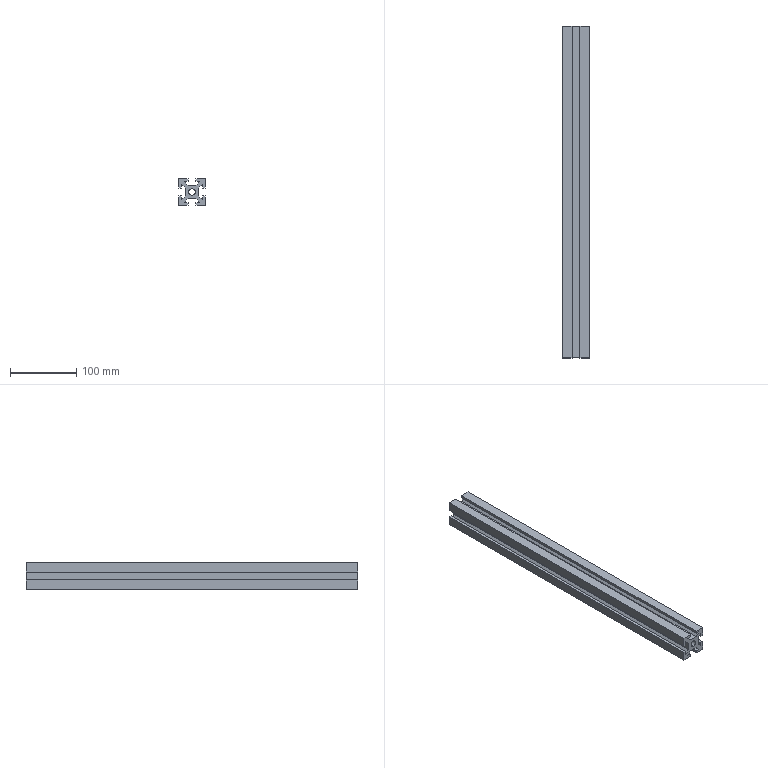Part | SolidWorks | features Extrusion 1 | 1 solid | 40 faces | box 40 x 500 x 40 mm | volume 454553 mm3 | plane 38 | cylinder 2 | commonest cylinder face diameters 10 x2
STEP:
#1=CARTESIAN_POINT('',(0.,500.,-5.));
#2=VERTEX_POINT('',#1);
#3=CARTESIAN_POINT('',(0.,500.,5.));
#4=VERTEX_POINT('',#3);
#5=CARTESIAN_POINT('',(0.,500.,0.));
#6=DIRECTION('',(0.,1.,0.));
#7=DIRECTION('',(0.,0.,1.));
#8=AXIS2_PLACEMENT_3D('',#5,#6,#7);
#9=CIRCLE('',#8,5.);
#10=EDGE_CURVE('',#2,#4,#9,.T.);
#11=ORIENTED_EDGE('',*,*,#10,.T.);
#12=CARTESIAN_POINT('',(0.,0.,5.));
#13=VERTEX_POINT('',#12);
#14=CARTESIAN_POINT('',(0.,500.,5.));
#15=DIRECTION('',(0.,-1.,0.));
#16=VECTOR('',#15,1000.);
#17=LINE('',#14,#16);
#18=EDGE_CURVE('',#4,#13,#17,.T.);
#19=ORIENTED_EDGE('',*,*,#18,.T.);
#20=CARTESIAN_POINT('',(0.,0.,-5.));
#21=VERTEX_POINT('',#20);
#22=CARTESIAN_POINT('',(0.,0.,0.));
#23=DIRECTION('',(0.,1.,0.));
#24=DIRECTION('',(0.,0.,1.));
#25=AXIS2_PLACEMENT_3D('',#22,#23,#24);
#26=CIRCLE('',#25,5.);
#27=EDGE_CURVE('',#21,#13,#26,.T.);
#28=ORIENTED_EDGE('',*,*,#27,.F.);
#29=CARTESIAN_POINT('',(0.,500.,-5.));
#30=DIRECTION('',(0.,-1.,0.));
#31=VECTOR('',#30,1000.);
#32=LINE('',#29,#31);
#33=EDGE_CURVE('',#2,#21,#32,.T.);
#34=ORIENTED_EDGE('',*,*,#33,.F.);
#35=EDGE_LOOP('',(#11,#19,#28,#34));
#36=FACE_OUTER_BOUND('',#35,.T.);
#37=CARTESIAN_POINT('',(0.,500.,0.));
#38=DIRECTION('',(0.,-1.,0.));
#39=DIRECTION('',(0.,0.,-1.));
#40=AXIS2_PLACEMENT_3D('',#37,#38,#39);
#41=CYLINDRICAL_SURFACE('',#40,5.);
#42=ADVANCED_FACE('',(#36),#41,.F.);
#43=CARTESIAN_POINT('',(6.,500.,20.));
#44=VERTEX_POINT('',#43);
#45=CARTESIAN_POINT('',(20.,500.,20.));
#46=VERTEX_POINT('',#45);
#47=CARTESIAN_POINT('',(6.,500.,20.));
#48=DIRECTION('',(1.,0.,0.));
#49=VECTOR('',#48,1000.);
#50=LINE('',#47,#49);
#51=EDGE_CURVE('',#44,#46,#50,.T.);
#52=ORIENTED_EDGE('',*,*,#51,.T.);
#53=CARTESIAN_POINT('',(20.,500.,6.));
#54=VERTEX_POINT('',#53);
#55=CARTESIAN_POINT('',(20.,500.,6.));
#56=DIRECTION('',(0.,0.,-1.));
#57=VECTOR('',#56,1000.);
#58=LINE('',#55,#57);
#59=EDGE_CURVE('',#46,#54,#58,.T.);
#60=ORIENTED_EDGE('',*,*,#59,.T.);
#61=CARTESIAN_POINT('',(16.,500.,6.));
#62=VERTEX_POINT('',#61);
#63=CARTESIAN_POINT('',(16.,500.,6.));
#64=DIRECTION('',(-1.,0.,0.));
#65=VECTOR('',#64,1000.);
#66=LINE('',#63,#65);
#67=EDGE_CURVE('',#54,#62,#66,.T.);
#68=ORIENTED_EDGE('',*,*,#67,.T.);
#69=CARTESIAN_POINT('',(16.,500.,11.757));
#70=VERTEX_POINT('',#69);
#71=CARTESIAN_POINT('',(16.,500.,11.757));
#72=DIRECTION('',(0.,0.,1.));
#73=VECTOR('',#72,1000.);
#74=LINE('',#71,#73);
#75=EDGE_CURVE('',#62,#70,#74,.T.);
#76=ORIENTED_EDGE('',*,*,#75,.T.);
#77=CARTESIAN_POINT('',(10.,500.,5.757));
#78=VERTEX_POINT('',#77);
#79=CARTESIAN_POINT('',(10.,500.,5.757));
#80=DIRECTION('',(-0.7071,0.,-0.7071));
#81=VECTOR('',#80,1000.);
#82=LINE('',#79,#81);
#83=EDGE_CURVE('',#70,#78,#82,.T.);
#84=ORIENTED_EDGE('',*,*,#83,.T.);
#85=CARTESIAN_POINT('',(10.,500.,-5.757));
#86=VERTEX_POINT('',#85);
#87=CARTESIAN_POINT('',(10.,500.,5.757));
#88=DIRECTION('',(0.,0.,-1.));
#89=VECTOR('',#88,1000.);
#90=LINE('',#87,#89);
#91=EDGE_CURVE('',#78,#86,#90,.T.);
#92=ORIENTED_EDGE('',*,*,#91,.T.);
#93=CARTESIAN_POINT('',(16.,500.,-11.757));
#94=VERTEX_POINT('',#93);
#95=CARTESIAN_POINT('',(16.,500.,-11.757));
#96=DIRECTION('',(0.7071,0.,-0.7071));
#97=VECTOR('',#96,1000.);
#98=LINE('',#95,#97);
#99=EDGE_CURVE('',#86,#94,#98,.T.);
#100=ORIENTED_EDGE('',*,*,#99,.T.);
#101=CARTESIAN_POINT('',(16.,500.,-6.));
#102=VERTEX_POINT('',#101);
#103=CARTESIAN_POINT('',(16.,500.,-6.));
#104=DIRECTION('',(0.,0.,1.));
#105=VECTOR('',#104,1000.);
#106=LINE('',#103,#105);
#107=EDGE_CURVE('',#94,#102,#106,.T.);
#108=ORIENTED_EDGE('',*,*,#107,.T.);
#109=CARTESIAN_POINT('',(20.,500.,-6.));
#110=VERTEX_POINT('',#109);
#111=CARTESIAN_POINT('',(20.,500.,-6.));
#112=DIRECTION('',(1.,0.,0.));
#113=VECTOR('',#112,1000.);
#114=LINE('',#111,#113);
#115=EDGE_CURVE('',#102,#110,#114,.T.);
#116=ORIENTED_EDGE('',*,*,#115,.T.);
#117=CARTESIAN_POINT('',(20.,500.,-20.));
#118=VERTEX_POINT('',#117);
#119=CARTESIAN_POINT('',(20.,500.,-20.));
#120=DIRECTION('',(0.,0.,-1.));
#121=VECTOR('',#120,1000.);
#122=LINE('',#119,#121);
#123=EDGE_CURVE('',#110,#118,#122,.T.);
#124=ORIENTED_EDGE('',*,*,#123,.T.);
#125=CARTESIAN_POINT('',(6.,500.,-20.));
#126=VERTEX_POINT('',#125);
#127=CARTESIAN_POINT('',(6.,500.,-20.));
#128=DIRECTION('',(-1.,0.,0.));
#129=VECTOR('',#128,1000.);
#130=LINE('',#127,#129);
#131=EDGE_CURVE('',#118,#126,#130,.T.);
#132=ORIENTED_EDGE('',*,*,#131,.T.);
#133=CARTESIAN_POINT('',(6.,500.,-16.));
#134=VERTEX_POINT('',#133);
#135=CARTESIAN_POINT('',(6.,500.,-16.));
#136=DIRECTION('',(0.,0.,1.));
#137=VECTOR('',#136,1000.);
#138=LINE('',#135,#137);
#139=EDGE_CURVE('',#126,#134,#138,.T.);
#140=ORIENTED_EDGE('',*,*,#139,.T.);
#141=CARTESIAN_POINT('',(11.757,500.,-16.));
#142=VERTEX_POINT('',#141);
#143=CARTESIAN_POINT('',(11.757,500.,-16.));
#144=DIRECTION('',(1.,0.,0.));
#145=VECTOR('',#144,1000.);
#146=LINE('',#143,#145);
#147=EDGE_CURVE('',#134,#142,#146,.T.);
#148=ORIENTED_EDGE('',*,*,#147,.T.);
#149=CARTESIAN_POINT('',(5.757,500.,-10.));
#150=VERTEX_POINT('',#149);
#151=CARTESIAN_POINT('',(5.757,500.,-10.));
#152=DIRECTION('',(-0.7071,0.,0.7071));
#153=VECTOR('',#152,1000.);
#154=LINE('',#151,#153);
#155=EDGE_CURVE('',#142,#150,#154,.T.);
#156=ORIENTED_EDGE('',*,*,#155,.T.);
#157=CARTESIAN_POINT('',(-5.757,500.,-10.));
#158=VERTEX_POINT('',#157);
#159=CARTESIAN_POINT('',(-5.757,500.,-10.));
#160=DIRECTION('',(-1.,0.,0.));
#161=VECTOR('',#160,1000.);
#162=LINE('',#159,#161);
#163=EDGE_CURVE('',#150,#158,#162,.T.);
#164=ORIENTED_EDGE('',*,*,#163,.T.);
#165=CARTESIAN_POINT('',(-11.757,500.,-16.));
#166=VERTEX_POINT('',#165);
#167=CARTESIAN_POINT('',(-11.757,500.,-16.));
#168=DIRECTION('',(-0.7071,0.,-0.7071));
#169=VECTOR('',#168,1000.);
#170=LINE('',#167,#169);
#171=EDGE_CURVE('',#158,#166,#170,.T.);
#172=ORIENTED_EDGE('',*,*,#171,.T.);
#173=CARTESIAN_POINT('',(-6.,500.,-16.));
#174=VERTEX_POINT('',#173);
#175=CARTESIAN_POINT('',(-6.,500.,-16.));
#176=DIRECTION('',(1.,0.,0.));
#177=VECTOR('',#176,1000.);
#178=LINE('',#175,#177);
#179=EDGE_CURVE('',#166,#174,#178,.T.);
#180=ORIENTED_EDGE('',*,*,#179,.T.);
#181=CARTESIAN_POINT('',(-6.,500.,-20.));
#182=VERTEX_POINT('',#181);
#183=CARTESIAN_POINT('',(-6.,500.,-20.));
#184=DIRECTION('',(0.,0.,-1.));
#185=VECTOR('',#184,1000.);
#186=LINE('',#183,#185);
#187=EDGE_CURVE('',#174,#182,#186,.T.);
#188=ORIENTED_EDGE('',*,*,#187,.T.);
#189=CARTESIAN_POINT('',(-20.,500.,-20.));
#190=VERTEX_POINT('',#189);
#191=CARTESIAN_POINT('',(-20.,500.,-20.));
#192=DIRECTION('',(-1.,0.,0.));
#193=VECTOR('',#192,1000.);
#194=LINE('',#191,#193);
#195=EDGE_CURVE('',#182,#190,#194,.T.);
#196=ORIENTED_EDGE('',*,*,#195,.T.);
#197=CARTESIAN_POINT('',(-20.,500.,-6.));
#198=VERTEX_POINT('',#197);
#199=CARTESIAN_POINT('',(-20.,500.,-20.));
#200=DIRECTION('',(0.,0.,1.));
#201=VECTOR('',#200,1000.);
#202=LINE('',#199,#201);
#203=EDGE_CURVE('',#190,#198,#202,.T.);
#204=ORIENTED_EDGE('',*,*,#203,.T.);
#205=CARTESIAN_POINT('',(-16.,500.,-6.));
#206=VERTEX_POINT('',#205);
#207=CARTESIAN_POINT('',(-16.,500.,-6.));
#208=DIRECTION('',(1.,0.,0.));
#209=VECTOR('',#208,1000.);
#210=LINE('',#207,#209);
#211=EDGE_CURVE('',#198,#206,#210,.T.);
#212=ORIENTED_EDGE('',*,*,#211,.T.);
#213=CARTESIAN_POINT('',(-16.,500.,-11.757));
#214=VERTEX_POINT('',#213);
#215=CARTESIAN_POINT('',(-16.,500.,-11.757));
#216=DIRECTION('',(0.,0.,-1.));
#217=VECTOR('',#216,1000.);
#218=LINE('',#215,#217);
#219=EDGE_CURVE('',#206,#214,#218,.T.);
#220=ORIENTED_EDGE('',*,*,#219,.T.);
#221=CARTESIAN_POINT('',(-10.,500.,-5.757));
#222=VERTEX_POINT('',#221);
#223=CARTESIAN_POINT('',(-10.,500.,-5.757));
#224=DIRECTION('',(0.7071,0.,0.7071));
#225=VECTOR('',#224,1000.);
#226=LINE('',#223,#225);
#227=EDGE_CURVE('',#214,#222,#226,.T.);
#228=ORIENTED_EDGE('',*,*,#227,.T.);
#229=CARTESIAN_POINT('',(-10.,500.,5.757));
#230=VERTEX_POINT('',#229);
#231=CARTESIAN_POINT('',(-10.,500.,5.757));
#232=DIRECTION('',(0.,0.,1.));
#233=VECTOR('',#232,1000.);
#234=LINE('',#231,#233);
#235=EDGE_CURVE('',#222,#230,#234,.T.);
#236=ORIENTED_EDGE('',*,*,#235,.T.);
#237=CARTESIAN_POINT('',(-16.,500.,11.757));
#238=VERTEX_POINT('',#237);
#239=CARTESIAN_POINT('',(-16.,500.,11.757));
#240=DIRECTION('',(-0.7071,0.,0.7071));
#241=VECTOR('',#240,1000.);
#242=LINE('',#239,#241);
#243=EDGE_CURVE('',#230,#238,#242,.T.);
#244=ORIENTED_EDGE('',*,*,#243,.T.);
#245=CARTESIAN_POINT('',(-16.,500.,6.));
#246=VERTEX_POINT('',#245);
#247=CARTESIAN_POINT('',(-16.,500.,6.));
#248=DIRECTION('',(0.,0.,-1.));
#249=VECTOR('',#248,1000.);
#250=LINE('',#247,#249);
#251=EDGE_CURVE('',#238,#246,#250,.T.);
#252=ORIENTED_EDGE('',*,*,#251,.T.);
#253=CARTESIAN_POINT('',(-20.,500.,6.));
#254=VERTEX_POINT('',#253);
#255=CARTESIAN_POINT('',(-20.,500.,6.));
#256=DIRECTION('',(-1.,0.,0.));
#257=VECTOR('',#256,1000.);
#258=LINE('',#255,#257);
#259=EDGE_CURVE('',#246,#254,#258,.T.);
#260=ORIENTED_EDGE('',*,*,#259,.T.);
#261=CARTESIAN_POINT('',(-20.,500.,20.));
#262=VERTEX_POINT('',#261);
#263=CARTESIAN_POINT('',(-20.,500.,6.));
#264=DIRECTION('',(0.,0.,1.));
#265=VECTOR('',#264,1000.);
#266=LINE('',#263,#265);
#267=EDGE_CURVE('',#254,#262,#266,.T.);
#268=ORIENTED_EDGE('',*,*,#267,.T.);
#269=CARTESIAN_POINT('',(-6.,500.,20.));
#270=VERTEX_POINT('',#269);
#271=CARTESIAN_POINT('',(-20.,500.,20.));
#272=DIRECTION('',(1.,0.,0.));
#273=VECTOR('',#272,1000.);
#274=LINE('',#271,#273);
#275=EDGE_CURVE('',#262,#270,#274,.T.);
#276=ORIENTED_EDGE('',*,*,#275,.T.);
#277=CARTESIAN_POINT('',(-6.,500.,16.));
#278=VERTEX_POINT('',#277);
#279=CARTESIAN_POINT('',(-6.,500.,16.));
#280=DIRECTION('',(0.,0.,-1.));
#281=VECTOR('',#280,1000.);
#282=LINE('',#279,#281);
#283=EDGE_CURVE('',#270,#278,#282,.T.);
#284=ORIENTED_EDGE('',*,*,#283,.T.);
#285=CARTESIAN_POINT('',(-11.757,500.,16.));
#286=VERTEX_POINT('',#285);
#287=CARTESIAN_POINT('',(-11.757,500.,16.));
#288=DIRECTION('',(-1.,0.,0.));
#289=VECTOR('',#288,1000.);
#290=LINE('',#287,#289);
#291=EDGE_CURVE('',#278,#286,#290,.T.);
#292=ORIENTED_EDGE('',*,*,#291,.T.);
#293=CARTESIAN_POINT('',(-5.757,500.,10.));
#294=VERTEX_POINT('',#293);
#295=CARTESIAN_POINT('',(-5.757,500.,10.));
#296=DIRECTION('',(0.7071,0.,-0.7071));
#297=VECTOR('',#296,1000.);
#298=LINE('',#295,#297);
#299=EDGE_CURVE('',#286,#294,#298,.T.);
#300=ORIENTED_EDGE('',*,*,#299,.T.);
#301=CARTESIAN_POINT('',(5.757,500.,10.));
#302=VERTEX_POINT('',#301);
#303=CARTESIAN_POINT('',(-5.757,500.,10.));
#304=DIRECTION('',(1.,0.,0.));
#305=VECTOR('',#304,1000.);
#306=LINE('',#303,#305);
#307=EDGE_CURVE('',#294,#302,#306,.T.);
#308=ORIENTED_EDGE('',*,*,#307,.T.);
#309=CARTESIAN_POINT('',(11.757,500.,16.));
#310=VERTEX_POINT('',#309);
#311=CARTESIAN_POINT('',(11.757,500.,16.));
#312=DIRECTION('',(0.7071,0.,0.7071));
#313=VECTOR('',#312,1000.);
#314=LINE('',#311,#313);
#315=EDGE_CURVE('',#302,#310,#314,.T.);
#316=ORIENTED_EDGE('',*,*,#315,.T.);
#317=CARTESIAN_POINT('',(6.,500.,16.));
#318=VERTEX_POINT('',#317);
#319=CARTESIAN_POINT('',(6.,500.,16.));
#320=DIRECTION('',(-1.,0.,0.));
#321=VECTOR('',#320,1000.);
#322=LINE('',#319,#321);
#323=EDGE_CURVE('',#310,#318,#322,.T.);
#324=ORIENTED_EDGE('',*,*,#323,.T.);
#325=CARTESIAN_POINT('',(6.,500.,20.));
#326=DIRECTION('',(0.,0.,1.));
#327=VECTOR('',#326,1000.);
#328=LINE('',#325,#327);
#329=EDGE_CURVE('',#318,#44,#328,.T.);
#330=ORIENTED_EDGE('',*,*,#329,.T.);
#331=EDGE_LOOP('',(#52,#60,#68,#76,#84,#92,#100,#108,#116,#124,#132,#140,#148,#156,#164,#172,#180,#188,#196,#204,#212,#220,#228,#236,#244,#252,#260,#268,#276,#284,#292,#300,#308,#316,#324,#330));
#332=FACE_OUTER_BOUND('',#331,.T.);
#333=ORIENTED_EDGE('',*,*,#10,.F.);
#334=CARTESIAN_POINT('',(0.,500.,0.));
#335=DIRECTION('',(0.,1.,0.));
#336=DIRECTION('',(0.,0.,1.));
#337=AXIS2_PLACEMENT_3D('',#334,#335,#336);
#338=CIRCLE('',#337,5.);
#339=EDGE_CURVE('',#4,#2,#338,.T.);
#340=ORIENTED_EDGE('',*,*,#339,.F.);
#341=EDGE_LOOP('',(#333,#340));
#342=FACE_BOUND('',#341,.T.);
#343=CARTESIAN_POINT('',(0.,500.,0.));
#344=DIRECTION('',(0.,-1.,0.));
#345=DIRECTION('',(0.,0.,-1.));
#346=AXIS2_PLACEMENT_3D('',#343,#344,#345);
#347=PLANE('',#346);
#348=ADVANCED_FACE('',(#332,#342),#347,.F.);
#349=CARTESIAN_POINT('',(6.,0.,20.));
#350=VERTEX_POINT('',#349);
#351=CARTESIAN_POINT('',(20.,0.,20.));
#352=VERTEX_POINT('',#351);
#353=CARTESIAN_POINT('',(6.,0.,20.));
#354=DIRECTION('',(1.,0.,0.));
#355=VECTOR('',#354,1000.);
#356=LINE('',#353,#355);
#357=EDGE_CURVE('',#350,#352,#356,.T.);
#358=ORIENTED_EDGE('',*,*,#357,.F.);
#359=CARTESIAN_POINT('',(6.,0.,16.));
#360=VERTEX_POINT('',#359);
#361=CARTESIAN_POINT('',(6.,0.,20.));
#362=DIRECTION('',(0.,0.,1.));
#363=VECTOR('',#362,1000.);
#364=LINE('',#361,#363);
#365=EDGE_CURVE('',#360,#350,#364,.T.);
#366=ORIENTED_EDGE('',*,*,#365,.F.);
#367=CARTESIAN_POINT('',(11.757,0.,16.));
#368=VERTEX_POINT('',#367);
#369=CARTESIAN_POINT('',(6.,0.,16.));
#370=DIRECTION('',(-1.,0.,0.));
#371=VECTOR('',#370,1000.);
#372=LINE('',#369,#371);
#373=EDGE_CURVE('',#368,#360,#372,.T.);
#374=ORIENTED_EDGE('',*,*,#373,.F.);
#375=CARTESIAN_POINT('',(5.757,0.,10.));
#376=VERTEX_POINT('',#375);
#377=CARTESIAN_POINT('',(11.757,0.,16.));
#378=DIRECTION('',(0.7071,0.,0.7071));
#379=VECTOR('',#378,1000.);
#380=LINE('',#377,#379);
#381=EDGE_CURVE('',#376,#368,#380,.T.);
#382=ORIENTED_EDGE('',*,*,#381,.F.);
#383=CARTESIAN_POINT('',(-5.757,0.,10.));
#384=VERTEX_POINT('',#383);
#385=CARTESIAN_POINT('',(-5.757,0.,10.));
#386=DIRECTION('',(1.,0.,0.));
#387=VECTOR('',#386,1000.);
#388=LINE('',#385,#387);
#389=EDGE_CURVE('',#384,#376,#388,.T.);
#390=ORIENTED_EDGE('',*,*,#389,.F.);
#391=CARTESIAN_POINT('',(-11.757,0.,16.));
#392=VERTEX_POINT('',#391);
#393=CARTESIAN_POINT('',(-5.757,0.,10.));
#394=DIRECTION('',(0.7071,0.,-0.7071));
#395=VECTOR('',#394,1000.);
#396=LINE('',#393,#395);
#397=EDGE_CURVE('',#392,#384,#396,.T.);
#398=ORIENTED_EDGE('',*,*,#397,.F.);
#399=CARTESIAN_POINT('',(-6.,0.,16.));
#400=VERTEX_POINT('',#399);
#401=CARTESIAN_POINT('',(-11.757,0.,16.));
#402=DIRECTION('',(-1.,0.,0.));
#403=VECTOR('',#402,1000.);
#404=LINE('',#401,#403);
#405=EDGE_CURVE('',#400,#392,#404,.T.);
#406=ORIENTED_EDGE('',*,*,#405,.F.);
#407=CARTESIAN_POINT('',(-6.,0.,20.));
#408=VERTEX_POINT('',#407);
#409=CARTESIAN_POINT('',(-6.,0.,16.));
#410=DIRECTION('',(0.,0.,-1.));
#411=VECTOR('',#410,1000.);
#412=LINE('',#409,#411);
#413=EDGE_CURVE('',#408,#400,#412,.T.);
#414=ORIENTED_EDGE('',*,*,#413,.F.);
#415=CARTESIAN_POINT('',(-20.,0.,20.));
#416=VERTEX_POINT('',#415);
#417=CARTESIAN_POINT('',(-20.,0.,20.));
#418=DIRECTION('',(1.,0.,0.));
#419=VECTOR('',#418,1000.);
#420=LINE('',#417,#419);
#421=EDGE_CURVE('',#416,#408,#420,.T.);
#422=ORIENTED_EDGE('',*,*,#421,.F.);
#423=CARTESIAN_POINT('',(-20.,0.,6.));
#424=VERTEX_POINT('',#423);
#425=CARTESIAN_POINT('',(-20.,0.,6.));
#426=DIRECTION('',(0.,0.,1.));
#427=VECTOR('',#426,1000.);
#428=LINE('',#425,#427);
#429=EDGE_CURVE('',#424,#416,#428,.T.);
#430=ORIENTED_EDGE('',*,*,#429,.F.);
#431=CARTESIAN_POINT('',(-16.,0.,6.));
#432=VERTEX_POINT('',#431);
#433=CARTESIAN_POINT('',(-20.,0.,6.));
#434=DIRECTION('',(-1.,0.,0.));
#435=VECTOR('',#434,1000.);
#436=LINE('',#433,#435);
#437=EDGE_CURVE('',#432,#424,#436,.T.);
#438=ORIENTED_EDGE('',*,*,#437,.F.);
#439=CARTESIAN_POINT('',(-16.,0.,11.757));
#440=VERTEX_POINT('',#439);
#441=CARTESIAN_POINT('',(-16.,0.,6.));
#442=DIRECTION('',(0.,0.,-1.));
#443=VECTOR('',#442,1000.);
#444=LINE('',#441,#443);
#445=EDGE_CURVE('',#440,#432,#444,.T.);
#446=ORIENTED_EDGE('',*,*,#445,.F.);
#447=CARTESIAN_POINT('',(-10.,0.,5.757));
#448=VERTEX_POINT('',#447);
#449=CARTESIAN_POINT('',(-16.,0.,11.757));
#450=DIRECTION('',(-0.7071,0.,0.7071));
#451=VECTOR('',#450,1000.);
#452=LINE('',#449,#451);
#453=EDGE_CURVE('',#448,#440,#452,.T.);
#454=ORIENTED_EDGE('',*,*,#453,.F.);
#455=CARTESIAN_POINT('',(-10.,0.,-5.757));
#456=VERTEX_POINT('',#455);
#457=CARTESIAN_POINT('',(-10.,0.,5.757));
#458=DIRECTION('',(0.,0.,1.));
#459=VECTOR('',#458,1000.);
#460=LINE('',#457,#459);
#461=EDGE_CURVE('',#456,#448,#460,.T.);
#462=ORIENTED_EDGE('',*,*,#461,.F.);
#463=CARTESIAN_POINT('',(-16.,0.,-11.757));
#464=VERTEX_POINT('',#463);
#465=CARTESIAN_POINT('',(-10.,0.,-5.757));
#466=DIRECTION('',(0.7071,0.,0.7071));
#467=VECTOR('',#466,1000.);
#468=LINE('',#465,#467);
#469=EDGE_CURVE('',#464,#456,#468,.T.);
#470=ORIENTED_EDGE('',*,*,#469,.F.);
#471=CARTESIAN_POINT('',(-16.,0.,-6.));
#472=VERTEX_POINT('',#471);
#473=CARTESIAN_POINT('',(-16.,0.,-11.757));
#474=DIRECTION('',(0.,0.,-1.));
#475=VECTOR('',#474,1000.);
#476=LINE('',#473,#475);
#477=EDGE_CURVE('',#472,#464,#476,.T.);
#478=ORIENTED_EDGE('',*,*,#477,.F.);
#479=CARTESIAN_POINT('',(-20.,0.,-6.));
#480=VERTEX_POINT('',#479);
#481=CARTESIAN_POINT('',(-16.,0.,-6.));
#482=DIRECTION('',(1.,0.,0.));
#483=VECTOR('',#482,1000.);
#484=LINE('',#481,#483);
#485=EDGE_CURVE('',#480,#472,#484,.T.);
#486=ORIENTED_EDGE('',*,*,#485,.F.);
#487=CARTESIAN_POINT('',(-20.,0.,-20.));
#488=VERTEX_POINT('',#487);
#489=CARTESIAN_POINT('',(-20.,0.,-20.));
#490=DIRECTION('',(0.,0.,1.));
#491=VECTOR('',#490,1000.);
#492=LINE('',#489,#491);
#493=EDGE_CURVE('',#488,#480,#492,.T.);
#494=ORIENTED_EDGE('',*,*,#493,.F.);
#495=CARTESIAN_POINT('',(-6.,0.,-20.));
#496=VERTEX_POINT('',#495);
#497=CARTESIAN_POINT('',(-20.,0.,-20.));
#498=DIRECTION('',(-1.,0.,0.));
#499=VECTOR('',#498,1000.);
#500=LINE('',#497,#499);
#501=EDGE_CURVE('',#496,#488,#500,.T.);
#502=ORIENTED_EDGE('',*,*,#501,.F.);
#503=CARTESIAN_POINT('',(-6.,0.,-16.));
#504=VERTEX_POINT('',#503);
#505=CARTESIAN_POINT('',(-6.,0.,-20.));
#506=DIRECTION('',(0.,0.,-1.));
#507=VECTOR('',#506,1000.);
#508=LINE('',#505,#507);
#509=EDGE_CURVE('',#504,#496,#508,.T.);
#510=ORIENTED_EDGE('',*,*,#509,.F.);
#511=CARTESIAN_POINT('',(-11.757,0.,-16.));
#512=VERTEX_POINT('',#511);
#513=CARTESIAN_POINT('',(-6.,0.,-16.));
#514=DIRECTION('',(1.,0.,0.));
#515=VECTOR('',#514,1000.);
#516=LINE('',#513,#515);
#517=EDGE_CURVE('',#512,#504,#516,.T.);
#518=ORIENTED_EDGE('',*,*,#517,.F.);
#519=CARTESIAN_POINT('',(-5.757,0.,-10.));
#520=VERTEX_POINT('',#519);
#521=CARTESIAN_POINT('',(-11.757,0.,-16.));
#522=DIRECTION('',(-0.7071,0.,-0.7071));
#523=VECTOR('',#522,1000.);
#524=LINE('',#521,#523);
#525=EDGE_CURVE('',#520,#512,#524,.T.);
#526=ORIENTED_EDGE('',*,*,#525,.F.);
#527=CARTESIAN_POINT('',(5.757,0.,-10.));
#528=VERTEX_POINT('',#527);
#529=CARTESIAN_POINT('',(-5.757,0.,-10.));
#530=DIRECTION('',(-1.,0.,0.));
#531=VECTOR('',#530,1000.);
#532=LINE('',#529,#531);
#533=EDGE_CURVE('',#528,#520,#532,.T.);
#534=ORIENTED_EDGE('',*,*,#533,.F.);
#535=CARTESIAN_POINT('',(11.757,0.,-16.));
#536=VERTEX_POINT('',#535);
#537=CARTESIAN_POINT('',(5.757,0.,-10.));
#538=DIRECTION('',(-0.7071,0.,0.7071));
#539=VECTOR('',#538,1000.);
#540=LINE('',#537,#539);
#541=EDGE_CURVE('',#536,#528,#540,.T.);
#542=ORIENTED_EDGE('',*,*,#541,.F.);
#543=CARTESIAN_POINT('',(6.,0.,-16.));
#544=VERTEX_POINT('',#543);
#545=CARTESIAN_POINT('',(11.757,0.,-16.));
#546=DIRECTION('',(1.,0.,0.));
#547=VECTOR('',#546,1000.);
#548=LINE('',#545,#547);
#549=EDGE_CURVE('',#544,#536,#548,.T.);
#550=ORIENTED_EDGE('',*,*,#549,.F.);
#551=CARTESIAN_POINT('',(6.,0.,-20.));
#552=VERTEX_POINT('',#551);
#553=CARTESIAN_POINT('',(6.,0.,-16.));
#554=DIRECTION('',(0.,0.,1.));
#555=VECTOR('',#554,1000.);
#556=LINE('',#553,#555);
#557=EDGE_CURVE('',#552,#544,#556,.T.);
#558=ORIENTED_EDGE('',*,*,#557,.F.);
#559=CARTESIAN_POINT('',(20.,0.,-20.));
#560=VERTEX_POINT('',#559);
#561=CARTESIAN_POINT('',(6.,0.,-20.));
#562=DIRECTION('',(-1.,0.,0.));
#563=VECTOR('',#562,1000.);
#564=LINE('',#561,#563);
#565=EDGE_CURVE('',#560,#552,#564,.T.);
#566=ORIENTED_EDGE('',*,*,#565,.F.);
#567=CARTESIAN_POINT('',(20.,0.,-6.));
#568=VERTEX_POINT('',#567);
#569=CARTESIAN_POINT('',(20.,0.,-20.));
#570=DIRECTION('',(0.,0.,-1.));
#571=VECTOR('',#570,1000.);
#572=LINE('',#569,#571);
#573=EDGE_CURVE('',#568,#560,#572,.T.);
#574=ORIENTED_EDGE('',*,*,#573,.F.);
#575=CARTESIAN_POINT('',(16.,0.,-6.));
#576=VERTEX_POINT('',#575);
#577=CARTESIAN_POINT('',(20.,0.,-6.));
#578=DIRECTION('',(1.,0.,0.));
#579=VECTOR('',#578,1000.);
#580=LINE('',#577,#579);
#581=EDGE_CURVE('',#576,#568,#580,.T.);
#582=ORIENTED_EDGE('',*,*,#581,.F.);
#583=CARTESIAN_POINT('',(16.,0.,-11.757));
#584=VERTEX_POINT('',#583);
#585=CARTESIAN_POINT('',(16.,0.,-6.));
#586=DIRECTION('',(0.,0.,1.));
#587=VECTOR('',#586,1000.);
#588=LINE('',#585,#587);
#589=EDGE_CURVE('',#584,#576,#588,.T.);
#590=ORIENTED_EDGE('',*,*,#589,.F.);
#591=CARTESIAN_POINT('',(10.,0.,-5.757));
#592=VERTEX_POINT('',#591);
#593=CARTESIAN_POINT('',(16.,0.,-11.757));
#594=DIRECTION('',(0.7071,0.,-0.7071));
#595=VECTOR('',#594,1000.);
#596=LINE('',#593,#595);
#597=EDGE_CURVE('',#592,#584,#596,.T.);
#598=ORIENTED_EDGE('',*,*,#597,.F.);
#599=CARTESIAN_POINT('',(10.,0.,5.757));
#600=VERTEX_POINT('',#599);
#601=CARTESIAN_POINT('',(10.,0.,5.757));
#602=DIRECTION('',(0.,0.,-1.));
#603=VECTOR('',#602,1000.);
#604=LINE('',#601,#603);
#605=EDGE_CURVE('',#600,#592,#604,.T.);
#606=ORIENTED_EDGE('',*,*,#605,.F.);
#607=CARTESIAN_POINT('',(16.,0.,11.757));
#608=VERTEX_POINT('',#607);
#609=CARTESIAN_POINT('',(10.,0.,5.757));
#610=DIRECTION('',(-0.7071,0.,-0.7071));
#611=VECTOR('',#610,1000.);
#612=LINE('',#609,#611);
#613=EDGE_CURVE('',#608,#600,#612,.T.);
#614=ORIENTED_EDGE('',*,*,#613,.F.);
#615=CARTESIAN_POINT('',(16.,0.,6.));
#616=VERTEX_POINT('',#615);
#617=CARTESIAN_POINT('',(16.,0.,11.757));
#618=DIRECTION('',(0.,0.,1.));
#619=VECTOR('',#618,1000.);
#620=LINE('',#617,#619);
#621=EDGE_CURVE('',#616,#608,#620,.T.);
#622=ORIENTED_EDGE('',*,*,#621,.F.);
#623=CARTESIAN_POINT('',(20.,0.,6.));
#624=VERTEX_POINT('',#623);
#625=CARTESIAN_POINT('',(16.,0.,6.));
#626=DIRECTION('',(-1.,0.,0.));
#627=VECTOR('',#626,1000.);
#628=LINE('',#625,#627);
#629=EDGE_CURVE('',#624,#616,#628,.T.);
#630=ORIENTED_EDGE('',*,*,#629,.F.);
#631=CARTESIAN_POINT('',(20.,0.,6.));
#632=DIRECTION('',(0.,0.,-1.));
#633=VECTOR('',#632,1000.);
#634=LINE('',#631,#633);
#635=EDGE_CURVE('',#352,#624,#634,.T.);
#636=ORIENTED_EDGE('',*,*,#635,.F.);
#637=EDGE_LOOP('',(#358,#366,#374,#382,#390,#398,#406,#414,#422,#430,#438,#446,#454,#462,#470,#478,#486,#494,#502,#510,#518,#526,#534,#542,#550,#558,#566,#574,#582,#590,#598,#606,#614,#622,#630,#636));
#638=FACE_OUTER_BOUND('',#637,.T.);
#639=ORIENTED_EDGE('',*,*,#27,.T.);
#640=CARTESIAN_POINT('',(0.,0.,0.));
#641=DIRECTION('',(0.,1.,0.));
#642=DIRECTION('',(0.,0.,1.));
#643=AXIS2_PLACEMENT_3D('',#640,#641,#642);
#644=CIRCLE('',#643,5.);
#645=EDGE_CURVE('',#13,#21,#644,.T.);
#646=ORIENTED_EDGE('',*,*,#645,.T.);
#647=EDGE_LOOP('',(#639,#646));
#648=FACE_BOUND('',#647,.T.);
#649=CARTESIAN_POINT('',(0.,0.,0.));
#650=DIRECTION('',(0.,-1.,0.));
#651=DIRECTION('',(0.,0.,-1.));
#652=AXIS2_PLACEMENT_3D('',#649,#650,#651);
#653=PLANE('',#652);
#654=ADVANCED_FACE('',(#638,#648),#653,.T.);
#655=ORIENTED_EDGE('',*,*,#357,.T.);
#656=CARTESIAN_POINT('',(20.,500.,20.));
#657=DIRECTION('',(0.,-1.,0.));
#658=VECTOR('',#657,1000.);
#659=LINE('',#656,#658);
#660=EDGE_CURVE('',#46,#352,#659,.T.);
#661=ORIENTED_EDGE('',*,*,#660,.F.);
#662=ORIENTED_EDGE('',*,*,#51,.F.);
#663=CARTESIAN_POINT('',(6.,500.,20.));
#664=DIRECTION('',(0.,-1.,0.));
#665=VECTOR('',#664,1000.);
#666=LINE('',#663,#665);
#667=EDGE_CURVE('',#44,#350,#666,.T.);
#668=ORIENTED_EDGE('',*,*,#667,.T.);
#669=EDGE_LOOP('',(#655,#661,#662,#668));
#670=FACE_OUTER_BOUND('',#669,.T.);
#671=CARTESIAN_POINT('',(6.,500.,20.));
#672=DIRECTION('',(0.,0.,-1.));
#673=DIRECTION('',(-1.,0.,0.));
#674=AXIS2_PLACEMENT_3D('',#671,#672,#673);
#675=PLANE('',#674);
#676=ADVANCED_FACE('',(#670),#675,.F.);
#677=ORIENTED_EDGE('',*,*,#635,.T.);
#678=CARTESIAN_POINT('',(20.,500.,6.));
#679=DIRECTION('',(0.,-1.,0.));
#680=VECTOR('',#679,1000.);
#681=LINE('',#678,#680);
#682=EDGE_CURVE('',#54,#624,#681,.T.);
#683=ORIENTED_EDGE('',*,*,#682,.F.);
#684=ORIENTED_EDGE('',*,*,#59,.F.);
#685=ORIENTED_EDGE('',*,*,#660,.T.);
#686=EDGE_LOOP('',(#677,#683,#684,#685));
#687=FACE_OUTER_BOUND('',#686,.T.);
#688=CARTESIAN_POINT('',(20.,500.,6.));
#689=DIRECTION('',(-1.,0.,0.));
#690=DIRECTION('',(0.,0.,1.));
#691=AXIS2_PLACEMENT_3D('',#688,#689,#690);
#692=PLANE('',#691);
#693=ADVANCED_FACE('',(#687),#692,.F.);
#694=ORIENTED_EDGE('',*,*,#629,.T.);
#695=CARTESIAN_POINT('',(16.,500.,6.));
#696=DIRECTION('',(0.,-1.,0.));
#697=VECTOR('',#696,1000.);
#698=LINE('',#695,#697);
#699=EDGE_CURVE('',#62,#616,#698,.T.);
#700=ORIENTED_EDGE('',*,*,#699,.F.);
#701=ORIENTED_EDGE('',*,*,#67,.F.);
#702=ORIENTED_EDGE('',*,*,#682,.T.);
#703=EDGE_LOOP('',(#694,#700,#701,#702));
#704=FACE_OUTER_BOUND('',#703,.T.);
#705=CARTESIAN_POINT('',(16.,500.,6.));
#706=DIRECTION('',(0.,0.,1.));
#707=DIRECTION('',(1.,0.,0.));
#708=AXIS2_PLACEMENT_3D('',#705,#706,#707);
#709=PLANE('',#708);
#710=ADVANCED_FACE('',(#704),#709,.F.);
#711=ORIENTED_EDGE('',*,*,#621,.T.);
#712=CARTESIAN_POINT('',(16.,500.,11.757));
#713=DIRECTION('',(0.,-1.,0.));
#714=VECTOR('',#713,1000.);
#715=LINE('',#712,#714);
#716=EDGE_CURVE('',#70,#608,#715,.T.);
#717=ORIENTED_EDGE('',*,*,#716,.F.);
#718=ORIENTED_EDGE('',*,*,#75,.F.);
#719=ORIENTED_EDGE('',*,*,#699,.T.);
#720=EDGE_LOOP('',(#711,#717,#718,#719));
#721=FACE_OUTER_BOUND('',#720,.T.);
#722=CARTESIAN_POINT('',(16.,500.,11.757));
#723=DIRECTION('',(1.,0.,0.));
#724=DIRECTION('',(0.,0.,-1.));
#725=AXIS2_PLACEMENT_3D('',#722,#723,#724);
#726=PLANE('',#725);
#727=ADVANCED_FACE('',(#721),#726,.F.);
#728=ORIENTED_EDGE('',*,*,#613,.T.);
#729=CARTESIAN_POINT('',(10.,500.,5.757));
#730=DIRECTION('',(0.,-1.,0.));
#731=VECTOR('',#730,1000.);
#732=LINE('',#729,#731);
#733=EDGE_CURVE('',#78,#600,#732,.T.);
#734=ORIENTED_EDGE('',*,*,#733,.F.);
#735=ORIENTED_EDGE('',*,*,#83,.F.);
#736=ORIENTED_EDGE('',*,*,#716,.T.);
#737=EDGE_LOOP('',(#728,#734,#735,#736));
#738=FACE_OUTER_BOUND('',#737,.T.);
#739=CARTESIAN_POINT('',(10.,500.,5.757));
#740=DIRECTION('',(-0.7071,0.,0.7071));
#741=DIRECTION('',(0.7071,0.,0.7071));
#742=AXIS2_PLACEMENT_3D('',#739,#740,#741);
#743=PLANE('',#742);
#744=ADVANCED_FACE('',(#738),#743,.F.);
#745=ORIENTED_EDGE('',*,*,#605,.T.);
#746=CARTESIAN_POINT('',(10.,500.,-5.757));
#747=DIRECTION('',(0.,-1.,0.));
#748=VECTOR('',#747,1000.);
#749=LINE('',#746,#748);
#750=EDGE_CURVE('',#86,#592,#749,.T.);
#751=ORIENTED_EDGE('',*,*,#750,.F.);
#752=ORIENTED_EDGE('',*,*,#91,.F.);
#753=ORIENTED_EDGE('',*,*,#733,.T.);
#754=EDGE_LOOP('',(#745,#751,#752,#753));
#755=FACE_OUTER_BOUND('',#754,.T.);
#756=CARTESIAN_POINT('',(10.,500.,5.757));
#757=DIRECTION('',(-1.,0.,0.));
#758=DIRECTION('',(0.,0.,1.));
#759=AXIS2_PLACEMENT_3D('',#756,#757,#758);
#760=PLANE('',#759);
#761=ADVANCED_FACE('',(#755),#760,.F.);
#762=ORIENTED_EDGE('',*,*,#597,.T.);
#763=CARTESIAN_POINT('',(16.,500.,-11.757));
#764=DIRECTION('',(0.,-1.,0.));
#765=VECTOR('',#764,1000.);
#766=LINE('',#763,#765);
#767=EDGE_CURVE('',#94,#584,#766,.T.);
#768=ORIENTED_EDGE('',*,*,#767,.F.);
#769=ORIENTED_EDGE('',*,*,#99,.F.);
#770=ORIENTED_EDGE('',*,*,#750,.T.);
#771=EDGE_LOOP('',(#762,#768,#769,#770));
#772=FACE_OUTER_BOUND('',#771,.T.);
#773=CARTESIAN_POINT('',(16.,500.,-11.757));
#774=DIRECTION('',(-0.7071,0.,-0.7071));
#775=DIRECTION('',(-0.7071,0.,0.7071));
#776=AXIS2_PLACEMENT_3D('',#773,#774,#775);
#777=PLANE('',#776);
#778=ADVANCED_FACE('',(#772),#777,.F.);
#779=ORIENTED_EDGE('',*,*,#589,.T.);
#780=CARTESIAN_POINT('',(16.,500.,-6.));
#781=DIRECTION('',(0.,-1.,0.));
#782=VECTOR('',#781,1000.);
#783=LINE('',#780,#782);
#784=EDGE_CURVE('',#102,#576,#783,.T.);
#785=ORIENTED_EDGE('',*,*,#784,.F.);
#786=ORIENTED_EDGE('',*,*,#107,.F.);
#787=ORIENTED_EDGE('',*,*,#767,.T.);
#788=EDGE_LOOP('',(#779,#785,#786,#787));
#789=FACE_OUTER_BOUND('',#788,.T.);
#790=CARTESIAN_POINT('',(16.,500.,-6.));
#791=DIRECTION('',(1.,0.,0.));
#792=DIRECTION('',(0.,0.,-1.));
#793=AXIS2_PLACEMENT_3D('',#790,#791,#792);
#794=PLANE('',#793);
#795=ADVANCED_FACE('',(#789),#794,.F.);
#796=ORIENTED_EDGE('',*,*,#581,.T.);
#797=CARTESIAN_POINT('',(20.,500.,-6.));
#798=DIRECTION('',(0.,-1.,0.));
#799=VECTOR('',#798,1000.);
#800=LINE('',#797,#799);
#801=EDGE_CURVE('',#110,#568,#800,.T.);
#802=ORIENTED_EDGE('',*,*,#801,.F.);
#803=ORIENTED_EDGE('',*,*,#115,.F.);
#804=ORIENTED_EDGE('',*,*,#784,.T.);
#805=EDGE_LOOP('',(#796,#802,#803,#804));
#806=FACE_OUTER_BOUND('',#805,.T.);
#807=CARTESIAN_POINT('',(20.,500.,-6.));
#808=DIRECTION('',(0.,0.,-1.));
#809=DIRECTION('',(-1.,0.,0.));
#810=AXIS2_PLACEMENT_3D('',#807,#808,#809);
#811=PLANE('',#810);
#812=ADVANCED_FACE('',(#806),#811,.F.);
#813=ORIENTED_EDGE('',*,*,#573,.T.);
#814=CARTESIAN_POINT('',(20.,500.,-20.));
#815=DIRECTION('',(0.,-1.,0.));
#816=VECTOR('',#815,1000.);
#817=LINE('',#814,#816);
#818=EDGE_CURVE('',#118,#560,#817,.T.);
#819=ORIENTED_EDGE('',*,*,#818,.F.);
#820=ORIENTED_EDGE('',*,*,#123,.F.);
#821=ORIENTED_EDGE('',*,*,#801,.T.);
#822=EDGE_LOOP('',(#813,#819,#820,#821));
#823=FACE_OUTER_BOUND('',#822,.T.);
#824=CARTESIAN_POINT('',(20.,500.,-20.));
#825=DIRECTION('',(-1.,0.,0.));
#826=DIRECTION('',(0.,0.,1.));
#827=AXIS2_PLACEMENT_3D('',#824,#825,#826);
#828=PLANE('',#827);
#829=ADVANCED_FACE('',(#823),#828,.F.);
#830=ORIENTED_EDGE('',*,*,#565,.T.);
#831=CARTESIAN_POINT('',(6.,500.,-20.));
#832=DIRECTION('',(0.,-1.,0.));
#833=VECTOR('',#832,1000.);
#834=LINE('',#831,#833);
#835=EDGE_CURVE('',#126,#552,#834,.T.);
#836=ORIENTED_EDGE('',*,*,#835,.F.);
#837=ORIENTED_EDGE('',*,*,#131,.F.);
#838=ORIENTED_EDGE('',*,*,#818,.T.);
#839=EDGE_LOOP('',(#830,#836,#837,#838));
#840=FACE_OUTER_BOUND('',#839,.T.);
#841=CARTESIAN_POINT('',(6.,500.,-20.));
#842=DIRECTION('',(0.,0.,1.));
#843=DIRECTION('',(1.,0.,0.));
#844=AXIS2_PLACEMENT_3D('',#841,#842,#843);
#845=PLANE('',#844);
#846=ADVANCED_FACE('',(#840),#845,.F.);
#847=ORIENTED_EDGE('',*,*,#557,.T.);
#848=CARTESIAN_POINT('',(6.,500.,-16.));
#849=DIRECTION('',(0.,-1.,0.));
#850=VECTOR('',#849,1000.);
#851=LINE('',#848,#850);
#852=EDGE_CURVE('',#134,#544,#851,.T.);
#853=ORIENTED_EDGE('',*,*,#852,.F.);
#854=ORIENTED_EDGE('',*,*,#139,.F.);
#855=ORIENTED_EDGE('',*,*,#835,.T.);
#856=EDGE_LOOP('',(#847,#853,#854,#855));
#857=FACE_OUTER_BOUND('',#856,.T.);
#858=CARTESIAN_POINT('',(6.,500.,-16.));
#859=DIRECTION('',(1.,0.,0.));
#860=DIRECTION('',(0.,0.,-1.));
#861=AXIS2_PLACEMENT_3D('',#858,#859,#860);
#862=PLANE('',#861);
#863=ADVANCED_FACE('',(#857),#862,.F.);
#864=ORIENTED_EDGE('',*,*,#549,.T.);
#865=CARTESIAN_POINT('',(11.757,500.,-16.));
#866=DIRECTION('',(0.,-1.,0.));
#867=VECTOR('',#866,1000.);
#868=LINE('',#865,#867);
#869=EDGE_CURVE('',#142,#536,#868,.T.);
#870=ORIENTED_EDGE('',*,*,#869,.F.);
#871=ORIENTED_EDGE('',*,*,#147,.F.);
#872=ORIENTED_EDGE('',*,*,#852,.T.);
#873=EDGE_LOOP('',(#864,#870,#871,#872));
#874=FACE_OUTER_BOUND('',#873,.T.);
#875=CARTESIAN_POINT('',(11.757,500.,-16.));
#876=DIRECTION('',(0.,0.,-1.));
#877=DIRECTION('',(-1.,0.,0.));
#878=AXIS2_PLACEMENT_3D('',#875,#876,#877);
#879=PLANE('',#878);
#880=ADVANCED_FACE('',(#874),#879,.F.);
#881=ORIENTED_EDGE('',*,*,#541,.T.);
#882=CARTESIAN_POINT('',(5.757,500.,-10.));
#883=DIRECTION('',(0.,-1.,0.));
#884=VECTOR('',#883,1000.);
#885=LINE('',#882,#884);
#886=EDGE_CURVE('',#150,#528,#885,.T.);
#887=ORIENTED_EDGE('',*,*,#886,.F.);
#888=ORIENTED_EDGE('',*,*,#155,.F.);
#889=ORIENTED_EDGE('',*,*,#869,.T.);
#890=EDGE_LOOP('',(#881,#887,#888,#889));
#891=FACE_OUTER_BOUND('',#890,.T.);
#892=CARTESIAN_POINT('',(5.757,500.,-10.));
#893=DIRECTION('',(0.7071,0.,0.7071));
#894=DIRECTION('',(0.7071,0.,-0.7071));
#895=AXIS2_PLACEMENT_3D('',#892,#893,#894);
#896=PLANE('',#895);
#897=ADVANCED_FACE('',(#891),#896,.F.);
#898=ORIENTED_EDGE('',*,*,#533,.T.);
#899=CARTESIAN_POINT('',(-5.757,500.,-10.));
#900=DIRECTION('',(0.,-1.,0.));
#901=VECTOR('',#900,1000.);
#902=LINE('',#899,#901);
#903=EDGE_CURVE('',#158,#520,#902,.T.);
#904=ORIENTED_EDGE('',*,*,#903,.F.);
#905=ORIENTED_EDGE('',*,*,#163,.F.);
#906=ORIENTED_EDGE('',*,*,#886,.T.);
#907=EDGE_LOOP('',(#898,#904,#905,#906));
#908=FACE_OUTER_BOUND('',#907,.T.);
#909=CARTESIAN_POINT('',(-5.757,500.,-10.));
#910=DIRECTION('',(0.,0.,1.));
#911=DIRECTION('',(1.,0.,0.));
#912=AXIS2_PLACEMENT_3D('',#909,#910,#911);
#913=PLANE('',#912);
#914=ADVANCED_FACE('',(#908),#913,.F.);
#915=ORIENTED_EDGE('',*,*,#525,.T.);
#916=CARTESIAN_POINT('',(-11.757,500.,-16.));
#917=DIRECTION('',(0.,-1.,0.));
#918=VECTOR('',#917,1000.);
#919=LINE('',#916,#918);
#920=EDGE_CURVE('',#166,#512,#919,.T.);
#921=ORIENTED_EDGE('',*,*,#920,.F.);
#922=ORIENTED_EDGE('',*,*,#171,.F.);
#923=ORIENTED_EDGE('',*,*,#903,.T.);
#924=EDGE_LOOP('',(#915,#921,#922,#923));
#925=FACE_OUTER_BOUND('',#924,.T.);
#926=CARTESIAN_POINT('',(-11.757,500.,-16.));
#927=DIRECTION('',(-0.7071,0.,0.7071));
#928=DIRECTION('',(0.7071,0.,0.7071));
#929=AXIS2_PLACEMENT_3D('',#926,#927,#928);
#930=PLANE('',#929);
#931=ADVANCED_FACE('',(#925),#930,.F.);
#932=ORIENTED_EDGE('',*,*,#517,.T.);
#933=CARTESIAN_POINT('',(-6.,500.,-16.));
#934=DIRECTION('',(0.,-1.,0.));
#935=VECTOR('',#934,1000.);
#936=LINE('',#933,#935);
#937=EDGE_CURVE('',#174,#504,#936,.T.);
#938=ORIENTED_EDGE('',*,*,#937,.F.);
#939=ORIENTED_EDGE('',*,*,#179,.F.);
#940=ORIENTED_EDGE('',*,*,#920,.T.);
#941=EDGE_LOOP('',(#932,#938,#939,#940));
#942=FACE_OUTER_BOUND('',#941,.T.);
#943=CARTESIAN_POINT('',(-6.,500.,-16.));
#944=DIRECTION('',(0.,0.,-1.));
#945=DIRECTION('',(-1.,0.,0.));
#946=AXIS2_PLACEMENT_3D('',#943,#944,#945);
#947=PLANE('',#946);
#948=ADVANCED_FACE('',(#942),#947,.F.);
#949=ORIENTED_EDGE('',*,*,#509,.T.);
#950=CARTESIAN_POINT('',(-6.,500.,-20.));
#951=DIRECTION('',(0.,-1.,0.));
#952=VECTOR('',#951,1000.);
#953=LINE('',#950,#952);
#954=EDGE_CURVE('',#182,#496,#953,.T.);
#955=ORIENTED_EDGE('',*,*,#954,.F.);
#956=ORIENTED_EDGE('',*,*,#187,.F.);
#957=ORIENTED_EDGE('',*,*,#937,.T.);
#958=EDGE_LOOP('',(#949,#955,#956,#957));
#959=FACE_OUTER_BOUND('',#958,.T.);
#960=CARTESIAN_POINT('',(-6.,500.,-20.));
#961=DIRECTION('',(-1.,0.,0.));
#962=DIRECTION('',(0.,0.,1.));
#963=AXIS2_PLACEMENT_3D('',#960,#961,#962);
#964=PLANE('',#963);
#965=ADVANCED_FACE('',(#959),#964,.F.);
#966=ORIENTED_EDGE('',*,*,#501,.T.);
#967=CARTESIAN_POINT('',(-20.,500.,-20.));
#968=DIRECTION('',(0.,-1.,0.));
#969=VECTOR('',#968,1000.);
#970=LINE('',#967,#969);
#971=EDGE_CURVE('',#190,#488,#970,.T.);
#972=ORIENTED_EDGE('',*,*,#971,.F.);
#973=ORIENTED_EDGE('',*,*,#195,.F.);
#974=ORIENTED_EDGE('',*,*,#954,.T.);
#975=EDGE_LOOP('',(#966,#972,#973,#974));
#976=FACE_OUTER_BOUND('',#975,.T.);
#977=CARTESIAN_POINT('',(-20.,500.,-20.));
#978=DIRECTION('',(0.,0.,1.));
#979=DIRECTION('',(1.,0.,0.));
#980=AXIS2_PLACEMENT_3D('',#977,#978,#979);
#981=PLANE('',#980);
#982=ADVANCED_FACE('',(#976),#981,.F.);
#983=ORIENTED_EDGE('',*,*,#493,.T.);
#984=CARTESIAN_POINT('',(-20.,500.,-6.));
#985=DIRECTION('',(0.,-1.,0.));
#986=VECTOR('',#985,1000.);
#987=LINE('',#984,#986);
#988=EDGE_CURVE('',#198,#480,#987,.T.);
#989=ORIENTED_EDGE('',*,*,#988,.F.);
#990=ORIENTED_EDGE('',*,*,#203,.F.);
#991=ORIENTED_EDGE('',*,*,#971,.T.);
#992=EDGE_LOOP('',(#983,#989,#990,#991));
#993=FACE_OUTER_BOUND('',#992,.T.);
#994=CARTESIAN_POINT('',(-20.,500.,-20.));
#995=DIRECTION('',(1.,0.,0.));
#996=DIRECTION('',(0.,0.,-1.));
#997=AXIS2_PLACEMENT_3D('',#994,#995,#996);
#998=PLANE('',#997);
#999=ADVANCED_FACE('',(#993),#998,.F.);
#1000=ORIENTED_EDGE('',*,*,#485,.T.);
#1001=CARTESIAN_POINT('',(-16.,500.,-6.));
#1002=DIRECTION('',(0.,-1.,0.));
#1003=VECTOR('',#1002,1000.);
#1004=LINE('',#1001,#1003);
#1005=EDGE_CURVE('',#206,#472,#1004,.T.);
#1006=ORIENTED_EDGE('',*,*,#1005,.F.);
#1007=ORIENTED_EDGE('',*,*,#211,.F.);
#1008=ORIENTED_EDGE('',*,*,#988,.T.);
#1009=EDGE_LOOP('',(#1000,#1006,#1007,#1008));
#1010=FACE_OUTER_BOUND('',#1009,.T.);
#1011=CARTESIAN_POINT('',(-16.,500.,-6.));
#1012=DIRECTION('',(0.,0.,-1.));
#1013=DIRECTION('',(-1.,0.,0.));
#1014=AXIS2_PLACEMENT_3D('',#1011,#1012,#1013);
#1015=PLANE('',#1014);
#1016=ADVANCED_FACE('',(#1010),#1015,.F.);
#1017=ORIENTED_EDGE('',*,*,#477,.T.);
#1018=CARTESIAN_POINT('',(-16.,500.,-11.757));
#1019=DIRECTION('',(0.,-1.,0.));
#1020=VECTOR('',#1019,1000.);
#1021=LINE('',#1018,#1020);
#1022=EDGE_CURVE('',#214,#464,#1021,.T.);
#1023=ORIENTED_EDGE('',*,*,#1022,.F.);
#1024=ORIENTED_EDGE('',*,*,#219,.F.);
#1025=ORIENTED_EDGE('',*,*,#1005,.T.);
#1026=EDGE_LOOP('',(#1017,#1023,#1024,#1025));
#1027=FACE_OUTER_BOUND('',#1026,.T.);
#1028=CARTESIAN_POINT('',(-16.,500.,-11.757));
#1029=DIRECTION('',(-1.,0.,0.));
#1030=DIRECTION('',(0.,0.,1.));
#1031=AXIS2_PLACEMENT_3D('',#1028,#1029,#1030);
#1032=PLANE('',#1031);
#1033=ADVANCED_FACE('',(#1027),#1032,.F.);
#1034=ORIENTED_EDGE('',*,*,#469,.T.);
#1035=CARTESIAN_POINT('',(-10.,500.,-5.757));
#1036=DIRECTION('',(0.,-1.,0.));
#1037=VECTOR('',#1036,1000.);
#1038=LINE('',#1035,#1037);
#1039=EDGE_CURVE('',#222,#456,#1038,.T.);
#1040=ORIENTED_EDGE('',*,*,#1039,.F.);
#1041=ORIENTED_EDGE('',*,*,#227,.F.);
#1042=ORIENTED_EDGE('',*,*,#1022,.T.);
#1043=EDGE_LOOP('',(#1034,#1040,#1041,#1042));
#1044=FACE_OUTER_BOUND('',#1043,.T.);
#1045=CARTESIAN_POINT('',(-10.,500.,-5.757));
#1046=DIRECTION('',(0.7071,0.,-0.7071));
#1047=DIRECTION('',(-0.7071,0.,-0.7071));
#1048=AXIS2_PLACEMENT_3D('',#1045,#1046,#1047);
#1049=PLANE('',#1048);
#1050=ADVANCED_FACE('',(#1044),#1049,.F.);
#1051=ORIENTED_EDGE('',*,*,#461,.T.);
#1052=CARTESIAN_POINT('',(-10.,500.,5.757));
#1053=DIRECTION('',(0.,-1.,0.));
#1054=VECTOR('',#1053,1000.);
#1055=LINE('',#1052,#1054);
#1056=EDGE_CURVE('',#230,#448,#1055,.T.);
#1057=ORIENTED_EDGE('',*,*,#1056,.F.);
#1058=ORIENTED_EDGE('',*,*,#235,.F.);
#1059=ORIENTED_EDGE('',*,*,#1039,.T.);
#1060=EDGE_LOOP('',(#1051,#1057,#1058,#1059));
#1061=FACE_OUTER_BOUND('',#1060,.T.);
#1062=CARTESIAN_POINT('',(-10.,500.,5.757));
#1063=DIRECTION('',(1.,0.,0.));
#1064=DIRECTION('',(0.,0.,-1.));
#1065=AXIS2_PLACEMENT_3D('',#1062,#1063,#1064);
#1066=PLANE('',#1065);
#1067=ADVANCED_FACE('',(#1061),#1066,.F.);
#1068=ORIENTED_EDGE('',*,*,#453,.T.);
#1069=CARTESIAN_POINT('',(-16.,500.,11.757));
#1070=DIRECTION('',(0.,-1.,0.));
#1071=VECTOR('',#1070,1000.);
#1072=LINE('',#1069,#1071);
#1073=EDGE_CURVE('',#238,#440,#1072,.T.);
#1074=ORIENTED_EDGE('',*,*,#1073,.F.);
#1075=ORIENTED_EDGE('',*,*,#243,.F.);
#1076=ORIENTED_EDGE('',*,*,#1056,.T.);
#1077=EDGE_LOOP('',(#1068,#1074,#1075,#1076));
#1078=FACE_OUTER_BOUND('',#1077,.T.);
#1079=CARTESIAN_POINT('',(-16.,500.,11.757));
#1080=DIRECTION('',(0.7071,0.,0.7071));
#1081=DIRECTION('',(0.7071,0.,-0.7071));
#1082=AXIS2_PLACEMENT_3D('',#1079,#1080,#1081);
#1083=PLANE('',#1082);
#1084=ADVANCED_FACE('',(#1078),#1083,.F.);
#1085=ORIENTED_EDGE('',*,*,#445,.T.);
#1086=CARTESIAN_POINT('',(-16.,500.,6.));
#1087=DIRECTION('',(0.,-1.,0.));
#1088=VECTOR('',#1087,1000.);
#1089=LINE('',#1086,#1088);
#1090=EDGE_CURVE('',#246,#432,#1089,.T.);
#1091=ORIENTED_EDGE('',*,*,#1090,.F.);
#1092=ORIENTED_EDGE('',*,*,#251,.F.);
#1093=ORIENTED_EDGE('',*,*,#1073,.T.);
#1094=EDGE_LOOP('',(#1085,#1091,#1092,#1093));
#1095=FACE_OUTER_BOUND('',#1094,.T.);
#1096=CARTESIAN_POINT('',(-16.,500.,6.));
#1097=DIRECTION('',(-1.,0.,0.));
#1098=DIRECTION('',(0.,0.,1.));
#1099=AXIS2_PLACEMENT_3D('',#1096,#1097,#1098);
#1100=PLANE('',#1099);
#1101=ADVANCED_FACE('',(#1095),#1100,.F.);
#1102=ORIENTED_EDGE('',*,*,#437,.T.);
#1103=CARTESIAN_POINT('',(-20.,500.,6.));
#1104=DIRECTION('',(0.,-1.,0.));
#1105=VECTOR('',#1104,1000.);
#1106=LINE('',#1103,#1105);
#1107=EDGE_CURVE('',#254,#424,#1106,.T.);
#1108=ORIENTED_EDGE('',*,*,#1107,.F.);
#1109=ORIENTED_EDGE('',*,*,#259,.F.);
#1110=ORIENTED_EDGE('',*,*,#1090,.T.);
#1111=EDGE_LOOP('',(#1102,#1108,#1109,#1110));
#1112=FACE_OUTER_BOUND('',#1111,.T.);
#1113=CARTESIAN_POINT('',(-20.,500.,6.));
#1114=DIRECTION('',(0.,0.,1.));
#1115=DIRECTION('',(1.,0.,0.));
#1116=AXIS2_PLACEMENT_3D('',#1113,#1114,#1115);
#1117=PLANE('',#1116);
#1118=ADVANCED_FACE('',(#1112),#1117,.F.);
#1119=ORIENTED_EDGE('',*,*,#429,.T.);
#1120=CARTESIAN_POINT('',(-20.,500.,20.));
#1121=DIRECTION('',(0.,-1.,0.));
#1122=VECTOR('',#1121,1000.);
#1123=LINE('',#1120,#1122);
#1124=EDGE_CURVE('',#262,#416,#1123,.T.);
#1125=ORIENTED_EDGE('',*,*,#1124,.F.);
#1126=ORIENTED_EDGE('',*,*,#267,.F.);
#1127=ORIENTED_EDGE('',*,*,#1107,.T.);
#1128=EDGE_LOOP('',(#1119,#1125,#1126,#1127));
#1129=FACE_OUTER_BOUND('',#1128,.T.);
#1130=CARTESIAN_POINT('',(-20.,500.,6.));
#1131=DIRECTION('',(1.,0.,0.));
#1132=DIRECTION('',(0.,0.,-1.));
#1133=AXIS2_PLACEMENT_3D('',#1130,#1131,#1132);
#1134=PLANE('',#1133);
#1135=ADVANCED_FACE('',(#1129),#1134,.F.);
#1136=ORIENTED_EDGE('',*,*,#421,.T.);
#1137=CARTESIAN_POINT('',(-6.,500.,20.));
#1138=DIRECTION('',(0.,-1.,0.));
#1139=VECTOR('',#1138,1000.);
#1140=LINE('',#1137,#1139);
#1141=EDGE_CURVE('',#270,#408,#1140,.T.);
#1142=ORIENTED_EDGE('',*,*,#1141,.F.);
#1143=ORIENTED_EDGE('',*,*,#275,.F.);
#1144=ORIENTED_EDGE('',*,*,#1124,.T.);
#1145=EDGE_LOOP('',(#1136,#1142,#1143,#1144));
#1146=FACE_OUTER_BOUND('',#1145,.T.);
#1147=CARTESIAN_POINT('',(-20.,500.,20.));
#1148=DIRECTION('',(0.,0.,-1.));
#1149=DIRECTION('',(-1.,0.,0.));
#1150=AXIS2_PLACEMENT_3D('',#1147,#1148,#1149);
#1151=PLANE('',#1150);
#1152=ADVANCED_FACE('',(#1146),#1151,.F.);
#1153=ORIENTED_EDGE('',*,*,#413,.T.);
#1154=CARTESIAN_POINT('',(-6.,500.,16.));
#1155=DIRECTION('',(0.,-1.,0.));
#1156=VECTOR('',#1155,1000.);
#1157=LINE('',#1154,#1156);
#1158=EDGE_CURVE('',#278,#400,#1157,.T.);
#1159=ORIENTED_EDGE('',*,*,#1158,.F.);
#1160=ORIENTED_EDGE('',*,*,#283,.F.);
#1161=ORIENTED_EDGE('',*,*,#1141,.T.);
#1162=EDGE_LOOP('',(#1153,#1159,#1160,#1161));
#1163=FACE_OUTER_BOUND('',#1162,.T.);
#1164=CARTESIAN_POINT('',(-6.,500.,16.));
#1165=DIRECTION('',(-1.,0.,0.));
#1166=DIRECTION('',(0.,0.,1.));
#1167=AXIS2_PLACEMENT_3D('',#1164,#1165,#1166);
#1168=PLANE('',#1167);
#1169=ADVANCED_FACE('',(#1163),#1168,.F.);
#1170=ORIENTED_EDGE('',*,*,#405,.T.);
#1171=CARTESIAN_POINT('',(-11.757,500.,16.));
#1172=DIRECTION('',(0.,-1.,0.));
#1173=VECTOR('',#1172,1000.);
#1174=LINE('',#1171,#1173);
#1175=EDGE_CURVE('',#286,#392,#1174,.T.);
#1176=ORIENTED_EDGE('',*,*,#1175,.F.);
#1177=ORIENTED_EDGE('',*,*,#291,.F.);
#1178=ORIENTED_EDGE('',*,*,#1158,.T.);
#1179=EDGE_LOOP('',(#1170,#1176,#1177,#1178));
#1180=FACE_OUTER_BOUND('',#1179,.T.);
#1181=CARTESIAN_POINT('',(-11.757,500.,16.));
#1182=DIRECTION('',(0.,0.,1.));
#1183=DIRECTION('',(1.,0.,0.));
#1184=AXIS2_PLACEMENT_3D('',#1181,#1182,#1183);
#1185=PLANE('',#1184);
#1186=ADVANCED_FACE('',(#1180),#1185,.F.);
#1187=ORIENTED_EDGE('',*,*,#397,.T.);
#1188=CARTESIAN_POINT('',(-5.757,500.,10.));
#1189=DIRECTION('',(0.,-1.,0.));
#1190=VECTOR('',#1189,1000.);
#1191=LINE('',#1188,#1190);
#1192=EDGE_CURVE('',#294,#384,#1191,.T.);
#1193=ORIENTED_EDGE('',*,*,#1192,.F.);
#1194=ORIENTED_EDGE('',*,*,#299,.F.);
#1195=ORIENTED_EDGE('',*,*,#1175,.T.);
#1196=EDGE_LOOP('',(#1187,#1193,#1194,#1195));
#1197=FACE_OUTER_BOUND('',#1196,.T.);
#1198=CARTESIAN_POINT('',(-5.757,500.,10.));
#1199=DIRECTION('',(-0.7071,0.,-0.7071));
#1200=DIRECTION('',(-0.7071,0.,0.7071));
#1201=AXIS2_PLACEMENT_3D('',#1198,#1199,#1200);
#1202=PLANE('',#1201);
#1203=ADVANCED_FACE('',(#1197),#1202,.F.);
#1204=ORIENTED_EDGE('',*,*,#389,.T.);
#1205=CARTESIAN_POINT('',(5.757,500.,10.));
#1206=DIRECTION('',(0.,-1.,0.));
#1207=VECTOR('',#1206,1000.);
#1208=LINE('',#1205,#1207);
#1209=EDGE_CURVE('',#302,#376,#1208,.T.);
#1210=ORIENTED_EDGE('',*,*,#1209,.F.);
#1211=ORIENTED_EDGE('',*,*,#307,.F.);
#1212=ORIENTED_EDGE('',*,*,#1192,.T.);
#1213=EDGE_LOOP('',(#1204,#1210,#1211,#1212));
#1214=FACE_OUTER_BOUND('',#1213,.T.);
#1215=CARTESIAN_POINT('',(-5.757,500.,10.));
#1216=DIRECTION('',(0.,0.,-1.));
#1217=DIRECTION('',(-1.,0.,0.));
#1218=AXIS2_PLACEMENT_3D('',#1215,#1216,#1217);
#1219=PLANE('',#1218);
#1220=ADVANCED_FACE('',(#1214),#1219,.F.);
#1221=ORIENTED_EDGE('',*,*,#381,.T.);
#1222=CARTESIAN_POINT('',(11.757,500.,16.));
#1223=DIRECTION('',(0.,-1.,0.));
#1224=VECTOR('',#1223,1000.);
#1225=LINE('',#1222,#1224);
#1226=EDGE_CURVE('',#310,#368,#1225,.T.);
#1227=ORIENTED_EDGE('',*,*,#1226,.F.);
#1228=ORIENTED_EDGE('',*,*,#315,.F.);
#1229=ORIENTED_EDGE('',*,*,#1209,.T.);
#1230=EDGE_LOOP('',(#1221,#1227,#1228,#1229));
#1231=FACE_OUTER_BOUND('',#1230,.T.);
#1232=CARTESIAN_POINT('',(11.757,500.,16.));
#1233=DIRECTION('',(0.7071,0.,-0.7071));
#1234=DIRECTION('',(-0.7071,0.,-0.7071));
#1235=AXIS2_PLACEMENT_3D('',#1232,#1233,#1234);
#1236=PLANE('',#1235);
#1237=ADVANCED_FACE('',(#1231),#1236,.F.);
#1238=ORIENTED_EDGE('',*,*,#373,.T.);
#1239=CARTESIAN_POINT('',(6.,500.,16.));
#1240=DIRECTION('',(0.,-1.,0.));
#1241=VECTOR('',#1240,1000.);
#1242=LINE('',#1239,#1241);
#1243=EDGE_CURVE('',#318,#360,#1242,.T.);
#1244=ORIENTED_EDGE('',*,*,#1243,.F.);
#1245=ORIENTED_EDGE('',*,*,#323,.F.);
#1246=ORIENTED_EDGE('',*,*,#1226,.T.);
#1247=EDGE_LOOP('',(#1238,#1244,#1245,#1246));
#1248=FACE_OUTER_BOUND('',#1247,.T.);
#1249=CARTESIAN_POINT('',(6.,500.,16.));
#1250=DIRECTION('',(0.,0.,1.));
#1251=DIRECTION('',(1.,0.,0.));
#1252=AXIS2_PLACEMENT_3D('',#1249,#1250,#1251);
#1253=PLANE('',#1252);
#1254=ADVANCED_FACE('',(#1248),#1253,.F.);
#1255=ORIENTED_EDGE('',*,*,#365,.T.);
#1256=ORIENTED_EDGE('',*,*,#667,.F.);
#1257=ORIENTED_EDGE('',*,*,#329,.F.);
#1258=ORIENTED_EDGE('',*,*,#1243,.T.);
#1259=EDGE_LOOP('',(#1255,#1256,#1257,#1258));
#1260=FACE_OUTER_BOUND('',#1259,.T.);
#1261=CARTESIAN_POINT('',(6.,500.,20.));
#1262=DIRECTION('',(1.,0.,0.));
#1263=DIRECTION('',(0.,0.,-1.));
#1264=AXIS2_PLACEMENT_3D('',#1261,#1262,#1263);
#1265=PLANE('',#1264);
#1266=ADVANCED_FACE('',(#1260),#1265,.F.);
#1267=ORIENTED_EDGE('',*,*,#18,.F.);
#1268=ORIENTED_EDGE('',*,*,#339,.T.);
#1269=ORIENTED_EDGE('',*,*,#33,.T.);
#1270=ORIENTED_EDGE('',*,*,#645,.F.);
#1271=EDGE_LOOP('',(#1267,#1268,#1269,#1270));
#1272=FACE_OUTER_BOUND('',#1271,.T.);
#1273=CARTESIAN_POINT('',(0.,500.,0.));
#1274=DIRECTION('',(0.,-1.,0.));
#1275=DIRECTION('',(0.,0.,-1.));
#1276=AXIS2_PLACEMENT_3D('',#1273,#1274,#1275);
#1277=CYLINDRICAL_SURFACE('',#1276,5.);
#1278=ADVANCED_FACE('',(#1272),#1277,.F.);
#1279=CLOSED_SHELL('',(#42,#348,#654,#676,#693,#710,#727,#744,#761,#778,#795,#812,#829,#846,#863,#880,#897,#914,#931,#948,#965,#982,#999,#1016,#1033,#1050,#1067,#1084,#1101,#1118,#1135,#1152,#1169,#1186,#1203,#1220,#1237,#1254,#1266,#1278));
#1280=MANIFOLD_SOLID_BREP('',#1279);
#1281=CARTESIAN_POINT('',(0.,0.,0.));
#1282=DIRECTION('',(0.,0.,1.));
#1283=DIRECTION('',(1.,0.,0.));
#1284=AXIS2_PLACEMENT_3D('',#1281,#1282,#1283);
#1285=(LENGTH_UNIT()NAMED_UNIT(*)SI_UNIT(.MILLI.,.METRE.));
#1286=UNCERTAINTY_MEASURE_WITH_UNIT(LENGTH_MEASURE(0.00001),#1285,'','');
#1287=(NAMED_UNIT(*)PLANE_ANGLE_UNIT()SI_UNIT($,.RADIAN.));
#1288=(NAMED_UNIT(*)SI_UNIT($,.STERADIAN.)SOLID_ANGLE_UNIT());
#1289=(GEOMETRIC_REPRESENTATION_CONTEXT(3)GLOBAL_UNCERTAINTY_ASSIGNED_CONTEXT((#1286))GLOBAL_UNIT_ASSIGNED_CONTEXT((#1285,#1287,#1288))REPRESENTATION_CONTEXT('',''));
#1290=ADVANCED_BREP_SHAPE_REPRESENTATION('',(#1280,#1284),#1289);